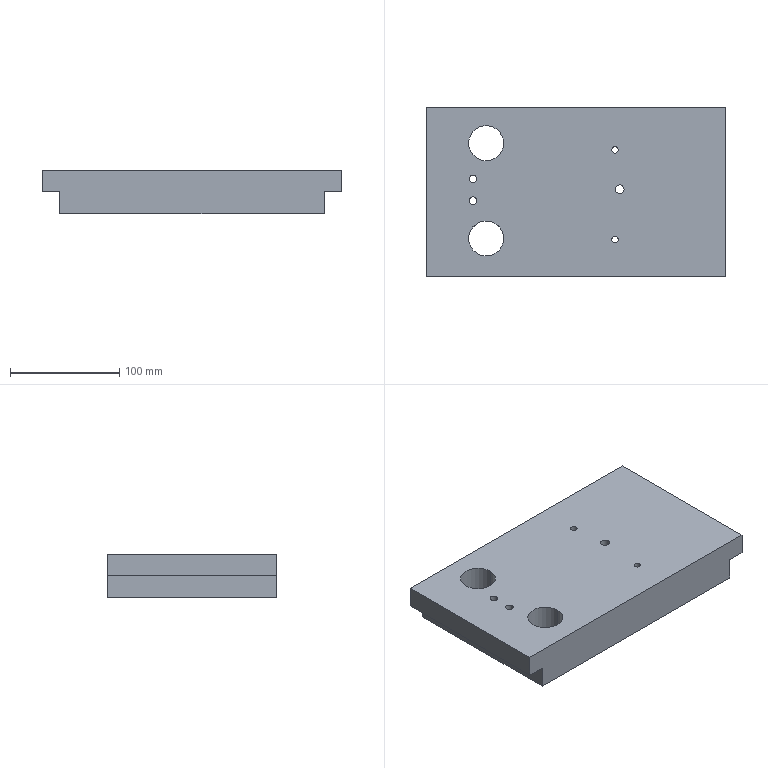Part | 1 solid | 48 faces | box 273.935 x 155 x 40 mm | volume 1346386 mm3 | cylinder 24 | plane 16 | cone 8 | commonest cylinder face diameters 8 x10 6 x4 7 x4 32 x4 34 x2